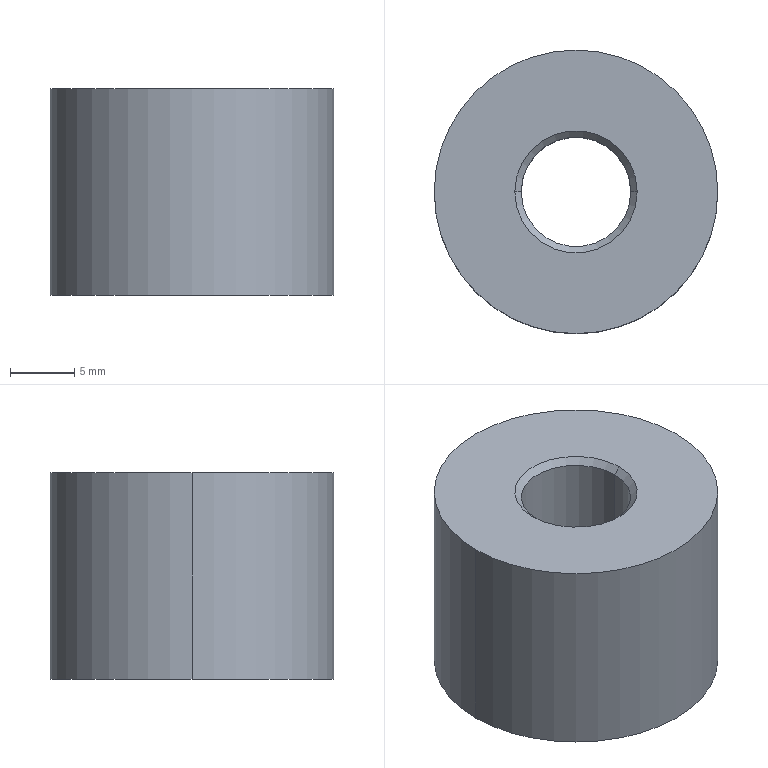Part | SolidWorks | features Chamfer 1, Extrusion 1, ICE 1 | 1 solid | 10 faces | box 22 x 22 x 16 mm | volume 5167 mm3 | cone 4 | cylinder 4 | plane 2 | commonest cylinder face diameters 8.5 x2 22 x2
STEP:
#1=CARTESIAN_POINT('',(-4.25,0.,15.5));
#2=VERTEX_POINT('',#1);
#3=CARTESIAN_POINT('',(4.25,0.,15.5));
#4=VERTEX_POINT('',#3);
#5=CARTESIAN_POINT('',(0.,0.,15.5));
#6=DIRECTION('',(0.,0.,1.));
#7=DIRECTION('',(1.,0.,0.));
#8=AXIS2_PLACEMENT_3D('',#5,#6,#7);
#9=CIRCLE('',#8,4.25);
#10=EDGE_CURVE('',#2,#4,#9,.T.);
#11=ORIENTED_EDGE('',*,*,#10,.F.);
#12=CARTESIAN_POINT('',(-4.75,0.,16.));
#13=VERTEX_POINT('',#12);
#14=CARTESIAN_POINT('',(-4.25,0.,15.5));
#15=DIRECTION('',(-0.7071,0.,0.7071));
#16=VECTOR('',#15,1000.);
#17=LINE('',#14,#16);
#18=EDGE_CURVE('',#2,#13,#17,.T.);
#19=ORIENTED_EDGE('',*,*,#18,.T.);
#20=CARTESIAN_POINT('',(4.75,0.,16.));
#21=VERTEX_POINT('',#20);
#22=CARTESIAN_POINT('',(0.,0.,16.));
#23=DIRECTION('',(0.,0.,-1.));
#24=DIRECTION('',(1.,0.,0.));
#25=AXIS2_PLACEMENT_3D('',#22,#23,#24);
#26=CIRCLE('',#25,4.75);
#27=EDGE_CURVE('',#21,#13,#26,.T.);
#28=ORIENTED_EDGE('',*,*,#27,.F.);
#29=CARTESIAN_POINT('',(4.25,0.,15.5));
#30=DIRECTION('',(0.7071,0.,0.7071));
#31=VECTOR('',#30,1000.);
#32=LINE('',#29,#31);
#33=EDGE_CURVE('',#4,#21,#32,.T.);
#34=ORIENTED_EDGE('',*,*,#33,.F.);
#35=EDGE_LOOP('',(#11,#19,#28,#34));
#36=FACE_OUTER_BOUND('',#35,.T.);
#37=CARTESIAN_POINT('',(0.,0.,15.5));
#38=DIRECTION('',(0.,0.,1.));
#39=DIRECTION('',(1.,0.,0.));
#40=AXIS2_PLACEMENT_3D('',#37,#38,#39);
#41=CONICAL_SURFACE('',#40,4.25,0.7854);
#42=ADVANCED_FACE('',(#36),#41,.F.);
#43=CARTESIAN_POINT('',(4.25,0.,0.5));
#44=VERTEX_POINT('',#43);
#45=CARTESIAN_POINT('',(-4.25,0.,0.5));
#46=VERTEX_POINT('',#45);
#47=CARTESIAN_POINT('',(0.,0.,0.5));
#48=DIRECTION('',(0.,0.,-1.));
#49=DIRECTION('',(1.,0.,0.));
#50=AXIS2_PLACEMENT_3D('',#47,#48,#49);
#51=CIRCLE('',#50,4.25);
#52=EDGE_CURVE('',#44,#46,#51,.T.);
#53=ORIENTED_EDGE('',*,*,#52,.F.);
#54=CARTESIAN_POINT('',(4.75,0.,0.));
#55=VERTEX_POINT('',#54);
#56=CARTESIAN_POINT('',(4.75,0.,0.));
#57=DIRECTION('',(0.7071,0.,-0.7071));
#58=VECTOR('',#57,1000.);
#59=LINE('',#56,#58);
#60=EDGE_CURVE('',#44,#55,#59,.T.);
#61=ORIENTED_EDGE('',*,*,#60,.T.);
#62=CARTESIAN_POINT('',(-4.75,0.,0.));
#63=VERTEX_POINT('',#62);
#64=CARTESIAN_POINT('',(0.,0.,0.));
#65=DIRECTION('',(0.,0.,1.));
#66=DIRECTION('',(1.,0.,0.));
#67=AXIS2_PLACEMENT_3D('',#64,#65,#66);
#68=CIRCLE('',#67,4.75);
#69=EDGE_CURVE('',#63,#55,#68,.T.);
#70=ORIENTED_EDGE('',*,*,#69,.F.);
#71=CARTESIAN_POINT('',(-4.75,0.,0.));
#72=DIRECTION('',(-0.7071,0.,-0.7071));
#73=VECTOR('',#72,1000.);
#74=LINE('',#71,#73);
#75=EDGE_CURVE('',#46,#63,#74,.T.);
#76=ORIENTED_EDGE('',*,*,#75,.F.);
#77=EDGE_LOOP('',(#53,#61,#70,#76));
#78=FACE_OUTER_BOUND('',#77,.T.);
#79=CARTESIAN_POINT('',(0.,0.,0.));
#80=DIRECTION('',(0.,0.,-1.));
#81=DIRECTION('',(-1.,0.,0.));
#82=AXIS2_PLACEMENT_3D('',#79,#80,#81);
#83=CONICAL_SURFACE('',#82,4.75,0.7854);
#84=ADVANCED_FACE('',(#78),#83,.F.);
#85=ORIENTED_EDGE('',*,*,#52,.T.);
#86=CARTESIAN_POINT('',(-4.25,0.,0.));
#87=DIRECTION('',(0.,0.,1.));
#88=VECTOR('',#87,1000.);
#89=LINE('',#86,#88);
#90=EDGE_CURVE('',#46,#2,#89,.T.);
#91=ORIENTED_EDGE('',*,*,#90,.T.);
#92=ORIENTED_EDGE('',*,*,#10,.T.);
#93=CARTESIAN_POINT('',(4.25,0.,0.));
#94=DIRECTION('',(0.,0.,1.));
#95=VECTOR('',#94,1000.);
#96=LINE('',#93,#95);
#97=EDGE_CURVE('',#44,#4,#96,.T.);
#98=ORIENTED_EDGE('',*,*,#97,.F.);
#99=EDGE_LOOP('',(#85,#91,#92,#98));
#100=FACE_OUTER_BOUND('',#99,.T.);
#101=CARTESIAN_POINT('',(0.,0.,0.));
#102=DIRECTION('',(0.,0.,1.));
#103=DIRECTION('',(1.,0.,0.));
#104=AXIS2_PLACEMENT_3D('',#101,#102,#103);
#105=CYLINDRICAL_SURFACE('',#104,4.25);
#106=ADVANCED_FACE('',(#100),#105,.F.);
#107=CARTESIAN_POINT('',(11.,0.,16.));
#108=VERTEX_POINT('',#107);
#109=CARTESIAN_POINT('',(-11.,0.,16.));
#110=VERTEX_POINT('',#109);
#111=CARTESIAN_POINT('',(0.,0.,16.));
#112=DIRECTION('',(0.,0.,1.));
#113=DIRECTION('',(1.,0.,0.));
#114=AXIS2_PLACEMENT_3D('',#111,#112,#113);
#115=CIRCLE('',#114,11.);
#116=EDGE_CURVE('',#108,#110,#115,.T.);
#117=ORIENTED_EDGE('',*,*,#116,.F.);
#118=CARTESIAN_POINT('',(11.,0.,0.));
#119=VERTEX_POINT('',#118);
#120=CARTESIAN_POINT('',(11.,0.,16.));
#121=DIRECTION('',(0.,0.,-1.));
#122=VECTOR('',#121,1000.);
#123=LINE('',#120,#122);
#124=EDGE_CURVE('',#108,#119,#123,.T.);
#125=ORIENTED_EDGE('',*,*,#124,.T.);
#126=CARTESIAN_POINT('',(-11.,0.,0.));
#127=VERTEX_POINT('',#126);
#128=CARTESIAN_POINT('',(0.,0.,0.));
#129=DIRECTION('',(0.,0.,1.));
#130=DIRECTION('',(1.,0.,0.));
#131=AXIS2_PLACEMENT_3D('',#128,#129,#130);
#132=CIRCLE('',#131,11.);
#133=EDGE_CURVE('',#119,#127,#132,.T.);
#134=ORIENTED_EDGE('',*,*,#133,.T.);
#135=CARTESIAN_POINT('',(-11.,0.,16.));
#136=DIRECTION('',(0.,0.,-1.));
#137=VECTOR('',#136,1000.);
#138=LINE('',#135,#137);
#139=EDGE_CURVE('',#110,#127,#138,.T.);
#140=ORIENTED_EDGE('',*,*,#139,.F.);
#141=EDGE_LOOP('',(#117,#125,#134,#140));
#142=FACE_OUTER_BOUND('',#141,.T.);
#143=CARTESIAN_POINT('',(0.,0.,16.));
#144=DIRECTION('',(0.,0.,-1.));
#145=DIRECTION('',(-1.,0.,0.));
#146=AXIS2_PLACEMENT_3D('',#143,#144,#145);
#147=CYLINDRICAL_SURFACE('',#146,11.);
#148=ADVANCED_FACE('',(#142),#147,.T.);
#149=ORIENTED_EDGE('',*,*,#124,.F.);
#150=CARTESIAN_POINT('',(0.,0.,16.));
#151=DIRECTION('',(0.,0.,1.));
#152=DIRECTION('',(1.,0.,0.));
#153=AXIS2_PLACEMENT_3D('',#150,#151,#152);
#154=CIRCLE('',#153,11.);
#155=EDGE_CURVE('',#110,#108,#154,.T.);
#156=ORIENTED_EDGE('',*,*,#155,.F.);
#157=ORIENTED_EDGE('',*,*,#139,.T.);
#158=CARTESIAN_POINT('',(0.,0.,0.));
#159=DIRECTION('',(0.,0.,1.));
#160=DIRECTION('',(1.,0.,0.));
#161=AXIS2_PLACEMENT_3D('',#158,#159,#160);
#162=CIRCLE('',#161,11.);
#163=EDGE_CURVE('',#127,#119,#162,.T.);
#164=ORIENTED_EDGE('',*,*,#163,.T.);
#165=EDGE_LOOP('',(#149,#156,#157,#164));
#166=FACE_OUTER_BOUND('',#165,.T.);
#167=CARTESIAN_POINT('',(0.,0.,16.));
#168=DIRECTION('',(0.,0.,-1.));
#169=DIRECTION('',(-1.,0.,0.));
#170=AXIS2_PLACEMENT_3D('',#167,#168,#169);
#171=CYLINDRICAL_SURFACE('',#170,11.);
#172=ADVANCED_FACE('',(#166),#171,.T.);
#173=ORIENTED_EDGE('',*,*,#27,.T.);
#174=CARTESIAN_POINT('',(0.,0.,16.));
#175=DIRECTION('',(0.,0.,-1.));
#176=DIRECTION('',(1.,0.,0.));
#177=AXIS2_PLACEMENT_3D('',#174,#175,#176);
#178=CIRCLE('',#177,4.75);
#179=EDGE_CURVE('',#13,#21,#178,.T.);
#180=ORIENTED_EDGE('',*,*,#179,.T.);
#181=EDGE_LOOP('',(#173,#180));
#182=FACE_BOUND('',#181,.T.);
#183=ORIENTED_EDGE('',*,*,#155,.T.);
#184=ORIENTED_EDGE('',*,*,#116,.T.);
#185=EDGE_LOOP('',(#183,#184));
#186=FACE_OUTER_BOUND('',#185,.T.);
#187=CARTESIAN_POINT('',(0.,0.,16.));
#188=DIRECTION('',(0.,0.,1.));
#189=DIRECTION('',(1.,0.,0.));
#190=AXIS2_PLACEMENT_3D('',#187,#188,#189);
#191=PLANE('',#190);
#192=ADVANCED_FACE('',(#182,#186),#191,.T.);
#193=ORIENTED_EDGE('',*,*,#69,.T.);
#194=CARTESIAN_POINT('',(0.,0.,0.));
#195=DIRECTION('',(0.,0.,1.));
#196=DIRECTION('',(1.,0.,0.));
#197=AXIS2_PLACEMENT_3D('',#194,#195,#196);
#198=CIRCLE('',#197,4.75);
#199=EDGE_CURVE('',#55,#63,#198,.T.);
#200=ORIENTED_EDGE('',*,*,#199,.T.);
#201=EDGE_LOOP('',(#193,#200));
#202=FACE_BOUND('',#201,.T.);
#203=ORIENTED_EDGE('',*,*,#163,.F.);
#204=ORIENTED_EDGE('',*,*,#133,.F.);
#205=EDGE_LOOP('',(#203,#204));
#206=FACE_OUTER_BOUND('',#205,.T.);
#207=CARTESIAN_POINT('',(0.,0.,0.));
#208=DIRECTION('',(0.,0.,1.));
#209=DIRECTION('',(1.,0.,0.));
#210=AXIS2_PLACEMENT_3D('',#207,#208,#209);
#211=PLANE('',#210);
#212=ADVANCED_FACE('',(#202,#206),#211,.F.);
#213=ORIENTED_EDGE('',*,*,#90,.F.);
#214=CARTESIAN_POINT('',(0.,0.,0.5));
#215=DIRECTION('',(0.,0.,-1.));
#216=DIRECTION('',(1.,0.,0.));
#217=AXIS2_PLACEMENT_3D('',#214,#215,#216);
#218=CIRCLE('',#217,4.25);
#219=EDGE_CURVE('',#46,#44,#218,.T.);
#220=ORIENTED_EDGE('',*,*,#219,.T.);
#221=ORIENTED_EDGE('',*,*,#97,.T.);
#222=CARTESIAN_POINT('',(0.,0.,15.5));
#223=DIRECTION('',(0.,0.,1.));
#224=DIRECTION('',(1.,0.,0.));
#225=AXIS2_PLACEMENT_3D('',#222,#223,#224);
#226=CIRCLE('',#225,4.25);
#227=EDGE_CURVE('',#4,#2,#226,.T.);
#228=ORIENTED_EDGE('',*,*,#227,.T.);
#229=EDGE_LOOP('',(#213,#220,#221,#228));
#230=FACE_OUTER_BOUND('',#229,.T.);
#231=CARTESIAN_POINT('',(0.,0.,0.));
#232=DIRECTION('',(0.,0.,1.));
#233=DIRECTION('',(1.,0.,0.));
#234=AXIS2_PLACEMENT_3D('',#231,#232,#233);
#235=CYLINDRICAL_SURFACE('',#234,4.25);
#236=ADVANCED_FACE('',(#230),#235,.F.);
#237=ORIENTED_EDGE('',*,*,#60,.F.);
#238=ORIENTED_EDGE('',*,*,#219,.F.);
#239=ORIENTED_EDGE('',*,*,#75,.T.);
#240=ORIENTED_EDGE('',*,*,#199,.F.);
#241=EDGE_LOOP('',(#237,#238,#239,#240));
#242=FACE_OUTER_BOUND('',#241,.T.);
#243=CARTESIAN_POINT('',(0.,0.,0.));
#244=DIRECTION('',(0.,0.,-1.));
#245=DIRECTION('',(-1.,0.,0.));
#246=AXIS2_PLACEMENT_3D('',#243,#244,#245);
#247=CONICAL_SURFACE('',#246,4.75,0.7854);
#248=ADVANCED_FACE('',(#242),#247,.F.);
#249=ORIENTED_EDGE('',*,*,#18,.F.);
#250=ORIENTED_EDGE('',*,*,#227,.F.);
#251=ORIENTED_EDGE('',*,*,#33,.T.);
#252=ORIENTED_EDGE('',*,*,#179,.F.);
#253=EDGE_LOOP('',(#249,#250,#251,#252));
#254=FACE_OUTER_BOUND('',#253,.T.);
#255=CARTESIAN_POINT('',(0.,0.,15.5));
#256=DIRECTION('',(0.,0.,1.));
#257=DIRECTION('',(1.,0.,0.));
#258=AXIS2_PLACEMENT_3D('',#255,#256,#257);
#259=CONICAL_SURFACE('',#258,4.25,0.7854);
#260=ADVANCED_FACE('',(#254),#259,.F.);
#261=CLOSED_SHELL('',(#42,#84,#106,#148,#172,#192,#212,#236,#248,#260));
#262=MANIFOLD_SOLID_BREP('',#261);
#263=CARTESIAN_POINT('',(0.,0.,0.));
#264=DIRECTION('',(0.,0.,1.));
#265=DIRECTION('',(1.,0.,0.));
#266=AXIS2_PLACEMENT_3D('',#263,#264,#265);
#267=(LENGTH_UNIT()NAMED_UNIT(*)SI_UNIT(.MILLI.,.METRE.));
#268=UNCERTAINTY_MEASURE_WITH_UNIT(LENGTH_MEASURE(0.00001),#267,'','');
#269=(NAMED_UNIT(*)PLANE_ANGLE_UNIT()SI_UNIT($,.RADIAN.));
#270=(NAMED_UNIT(*)SI_UNIT($,.STERADIAN.)SOLID_ANGLE_UNIT());
#271=(GEOMETRIC_REPRESENTATION_CONTEXT(3)GLOBAL_UNCERTAINTY_ASSIGNED_CONTEXT((#268))GLOBAL_UNIT_ASSIGNED_CONTEXT((#267,#269,#270))REPRESENTATION_CONTEXT('',''));
#272=ADVANCED_BREP_SHAPE_REPRESENTATION('',(#262,#266),#271);